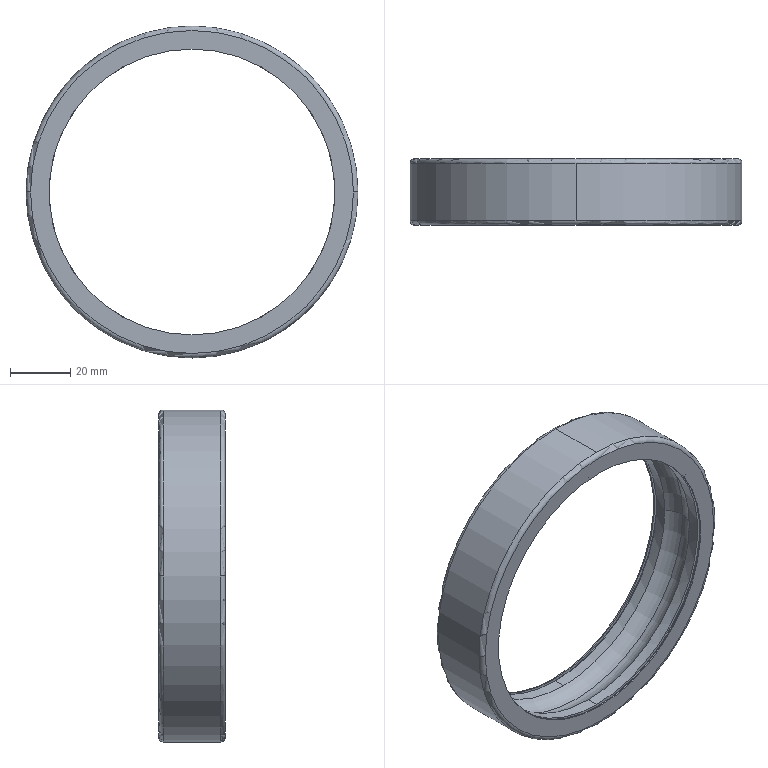Part | SolidWorks | features BaseBody 1 | 1 solid | 28 faces | box 110 x 22 x 110 mm | volume 46776 mm3 | cylinder 14 | torus 8 | plane 6 | commonest cylinder face diameters 94.7 x8 96.7 x4 110 x2
STEP:
#1=CARTESIAN_POINT('',(-2132.95,1024.569,-1530.274));
#2=VERTEX_POINT('',#1);
#3=CARTESIAN_POINT('',(-2132.95,1024.569,-1624.974));
#4=VERTEX_POINT('',#3);
#5=CARTESIAN_POINT('',(-2132.95,1024.569,-1577.624));
#6=DIRECTION('',(0.,-1.,0.));
#7=DIRECTION('',(0.,0.,1.));
#8=AXIS2_PLACEMENT_3D('',#5,#6,#7);
#9=CIRCLE('',#8,47.35);
#10=EDGE_CURVE('',#2,#4,#9,.T.);
#11=ORIENTED_EDGE('',*,*,#10,.F.);
#12=CARTESIAN_POINT('',(-2132.95,1024.569,-1577.624));
#13=DIRECTION('',(0.,-1.,0.));
#14=DIRECTION('',(0.,0.,-1.));
#15=AXIS2_PLACEMENT_3D('',#12,#13,#14);
#16=CIRCLE('',#15,47.35);
#17=EDGE_CURVE('',#4,#2,#16,.T.);
#18=ORIENTED_EDGE('',*,*,#17,.F.);
#19=EDGE_LOOP('',(#11,#18));
#20=FACE_BOUND('',#19,.T.);
#21=CARTESIAN_POINT('',(-2079.45,1024.569,-1577.624));
#22=VERTEX_POINT('',#21);
#23=CARTESIAN_POINT('',(-2186.45,1024.569,-1577.624));
#24=VERTEX_POINT('',#23);
#25=CARTESIAN_POINT('',(-2132.95,1024.569,-1577.624));
#26=DIRECTION('',(0.,-1.,0.));
#27=DIRECTION('',(0.,0.,1.));
#28=AXIS2_PLACEMENT_3D('',#25,#26,#27);
#29=CIRCLE('',#28,53.5);
#30=EDGE_CURVE('',#22,#24,#29,.T.);
#31=ORIENTED_EDGE('',*,*,#30,.T.);
#32=CARTESIAN_POINT('',(-2132.95,1024.569,-1577.624));
#33=DIRECTION('',(0.,-1.,0.));
#34=DIRECTION('',(-1.,0.,0.));
#35=AXIS2_PLACEMENT_3D('',#32,#33,#34);
#36=CIRCLE('',#35,53.5);
#37=EDGE_CURVE('',#24,#22,#36,.T.);
#38=ORIENTED_EDGE('',*,*,#37,.T.);
#39=EDGE_LOOP('',(#31,#38));
#40=FACE_OUTER_BOUND('',#39,.T.);
#41=CARTESIAN_POINT('',(-2074.1,1024.569,-1636.435));
#42=DIRECTION('',(0.,-1.,0.));
#43=DIRECTION('',(0.,0.,-1.));
#44=AXIS2_PLACEMENT_3D('',#41,#42,#43);
#45=PLANE('',#44);
#46=ADVANCED_FACE('',(#20,#40),#45,.T.);
#47=CARTESIAN_POINT('',(-2077.95,1026.069,-1577.624));
#48=VERTEX_POINT('',#47);
#49=CARTESIAN_POINT('',(-2079.45,1026.069,-1577.624));
#50=DIRECTION('',(0.,0.,-1.));
#51=DIRECTION('',(1.,0.,0.));
#52=AXIS2_PLACEMENT_3D('',#49,#50,#51);
#53=CIRCLE('',#52,1.5);
#54=EDGE_CURVE('',#48,#22,#53,.T.);
#55=ORIENTED_EDGE('',*,*,#54,.T.);
#56=ORIENTED_EDGE('',*,*,#37,.F.);
#57=CARTESIAN_POINT('',(-2187.95,1026.069,-1577.624));
#58=VERTEX_POINT('',#57);
#59=CARTESIAN_POINT('',(-2186.45,1026.069,-1577.624));
#60=DIRECTION('',(0.,0.,-1.));
#61=DIRECTION('',(0.,-1.,0.));
#62=AXIS2_PLACEMENT_3D('',#59,#60,#61);
#63=CIRCLE('',#62,1.5);
#64=EDGE_CURVE('',#24,#58,#63,.T.);
#65=ORIENTED_EDGE('',*,*,#64,.T.);
#66=CARTESIAN_POINT('',(-2132.95,1026.069,-1632.624));
#67=VERTEX_POINT('',#66);
#68=CARTESIAN_POINT('',(-2132.95,1026.069,-1577.624));
#69=DIRECTION('',(0.,-1.,0.));
#70=DIRECTION('',(-1.,0.,0.));
#71=AXIS2_PLACEMENT_3D('',#68,#69,#70);
#72=CIRCLE('',#71,55.);
#73=EDGE_CURVE('',#58,#67,#72,.T.);
#74=ORIENTED_EDGE('',*,*,#73,.T.);
#75=CARTESIAN_POINT('',(-2132.95,1026.069,-1577.624));
#76=DIRECTION('',(0.,-1.,0.));
#77=DIRECTION('',(0.,0.,-1.));
#78=AXIS2_PLACEMENT_3D('',#75,#76,#77);
#79=CIRCLE('',#78,55.);
#80=EDGE_CURVE('',#67,#48,#79,.T.);
#81=ORIENTED_EDGE('',*,*,#80,.T.);
#82=EDGE_LOOP('',(#55,#56,#65,#74,#81));
#83=FACE_OUTER_BOUND('',#82,.T.);
#84=CARTESIAN_POINT('',(-2132.95,1026.069,-1577.624));
#85=DIRECTION('',(0.,-1.,0.));
#86=DIRECTION('',(-0.9962,0.,0.08716));
#87=AXIS2_PLACEMENT_3D('',#84,#85,#86);
#88=TOROIDAL_SURFACE('',#87,53.5,1.5);
#89=ADVANCED_FACE('',(#83),#88,.T.);
#90=CARTESIAN_POINT('',(-2132.95,1045.069,-1522.624));
#91=VERTEX_POINT('',#90);
#92=CARTESIAN_POINT('',(-2132.95,1026.069,-1522.624));
#93=VERTEX_POINT('',#92);
#94=CARTESIAN_POINT('',(-2132.95,1045.069,-1522.624));
#95=DIRECTION('',(0.,-1.,0.));
#96=VECTOR('',#95,1000.);
#97=LINE('',#94,#96);
#98=EDGE_CURVE('',#91,#93,#97,.T.);
#99=ORIENTED_EDGE('',*,*,#98,.T.);
#100=CARTESIAN_POINT('',(-2132.95,1026.069,-1577.624));
#101=DIRECTION('',(0.,-1.,0.));
#102=DIRECTION('',(1.,0.,0.));
#103=AXIS2_PLACEMENT_3D('',#100,#101,#102);
#104=CIRCLE('',#103,55.);
#105=EDGE_CURVE('',#48,#93,#104,.T.);
#106=ORIENTED_EDGE('',*,*,#105,.F.);
#107=ORIENTED_EDGE('',*,*,#80,.F.);
#108=CARTESIAN_POINT('',(-2132.95,1045.069,-1632.624));
#109=VERTEX_POINT('',#108);
#110=CARTESIAN_POINT('',(-2132.95,1026.069,-1632.624));
#111=DIRECTION('',(0.,1.,0.));
#112=VECTOR('',#111,1000.);
#113=LINE('',#110,#112);
#114=EDGE_CURVE('',#67,#109,#113,.T.);
#115=ORIENTED_EDGE('',*,*,#114,.T.);
#116=CARTESIAN_POINT('',(-2077.95,1045.069,-1577.624));
#117=VERTEX_POINT('',#116);
#118=CARTESIAN_POINT('',(-2132.95,1045.069,-1577.624));
#119=DIRECTION('',(0.,-1.,0.));
#120=DIRECTION('',(0.,0.,-1.));
#121=AXIS2_PLACEMENT_3D('',#118,#119,#120);
#122=CIRCLE('',#121,55.);
#123=EDGE_CURVE('',#109,#117,#122,.T.);
#124=ORIENTED_EDGE('',*,*,#123,.T.);
#125=CARTESIAN_POINT('',(-2132.95,1045.069,-1577.624));
#126=DIRECTION('',(0.,-1.,0.));
#127=DIRECTION('',(1.,0.,0.));
#128=AXIS2_PLACEMENT_3D('',#125,#126,#127);
#129=CIRCLE('',#128,55.);
#130=EDGE_CURVE('',#117,#91,#129,.T.);
#131=ORIENTED_EDGE('',*,*,#130,.T.);
#132=EDGE_LOOP('',(#99,#106,#107,#115,#124,#131));
#133=FACE_OUTER_BOUND('',#132,.T.);
#134=CARTESIAN_POINT('',(-2132.95,1046.019,-1577.624));
#135=DIRECTION('',(0.,1.,0.));
#136=DIRECTION('',(-0.08716,0.,0.9962));
#137=AXIS2_PLACEMENT_3D('',#134,#135,#136);
#138=CYLINDRICAL_SURFACE('',#137,55.);
#139=ADVANCED_FACE('',(#133),#138,.T.);
#140=CARTESIAN_POINT('',(-2079.45,1046.569,-1577.624));
#141=VERTEX_POINT('',#140);
#142=CARTESIAN_POINT('',(-2079.45,1045.069,-1577.624));
#143=DIRECTION('',(0.,0.,-1.));
#144=DIRECTION('',(0.,1.,0.));
#145=AXIS2_PLACEMENT_3D('',#142,#143,#144);
#146=CIRCLE('',#145,1.5);
#147=EDGE_CURVE('',#141,#117,#146,.T.);
#148=ORIENTED_EDGE('',*,*,#147,.T.);
#149=ORIENTED_EDGE('',*,*,#123,.F.);
#150=CARTESIAN_POINT('',(-2187.95,1045.069,-1577.624));
#151=VERTEX_POINT('',#150);
#152=CARTESIAN_POINT('',(-2132.95,1045.069,-1577.624));
#153=DIRECTION('',(0.,-1.,0.));
#154=DIRECTION('',(-1.,0.,0.));
#155=AXIS2_PLACEMENT_3D('',#152,#153,#154);
#156=CIRCLE('',#155,55.);
#157=EDGE_CURVE('',#151,#109,#156,.T.);
#158=ORIENTED_EDGE('',*,*,#157,.F.);
#159=CARTESIAN_POINT('',(-2186.45,1046.569,-1577.624));
#160=VERTEX_POINT('',#159);
#161=CARTESIAN_POINT('',(-2186.45,1045.069,-1577.624));
#162=DIRECTION('',(0.,0.,-1.));
#163=DIRECTION('',(-1.,0.,0.));
#164=AXIS2_PLACEMENT_3D('',#161,#162,#163);
#165=CIRCLE('',#164,1.5);
#166=EDGE_CURVE('',#151,#160,#165,.T.);
#167=ORIENTED_EDGE('',*,*,#166,.T.);
#168=CARTESIAN_POINT('',(-2132.95,1046.569,-1577.624));
#169=DIRECTION('',(0.,1.,0.));
#170=DIRECTION('',(1.,0.,0.));
#171=AXIS2_PLACEMENT_3D('',#168,#169,#170);
#172=CIRCLE('',#171,53.5);
#173=EDGE_CURVE('',#141,#160,#172,.T.);
#174=ORIENTED_EDGE('',*,*,#173,.F.);
#175=EDGE_LOOP('',(#148,#149,#158,#167,#174));
#176=FACE_OUTER_BOUND('',#175,.T.);
#177=CARTESIAN_POINT('',(-2132.95,1045.069,-1577.624));
#178=DIRECTION('',(0.,-1.,0.));
#179=DIRECTION('',(-0.9962,0.,0.08716));
#180=AXIS2_PLACEMENT_3D('',#177,#178,#179);
#181=TOROIDAL_SURFACE('',#180,53.5,1.5);
#182=ADVANCED_FACE('',(#176),#181,.T.);
#183=CARTESIAN_POINT('',(-2132.95,1046.569,-1624.974));
#184=VERTEX_POINT('',#183);
#185=CARTESIAN_POINT('',(-2132.95,1046.569,-1530.274));
#186=VERTEX_POINT('',#185);
#187=CARTESIAN_POINT('',(-2132.95,1046.569,-1577.624));
#188=DIRECTION('',(0.,1.,0.));
#189=DIRECTION('',(0.,0.,-1.));
#190=AXIS2_PLACEMENT_3D('',#187,#188,#189);
#191=CIRCLE('',#190,47.35);
#192=EDGE_CURVE('',#184,#186,#191,.T.);
#193=ORIENTED_EDGE('',*,*,#192,.F.);
#194=CARTESIAN_POINT('',(-2132.95,1046.569,-1577.624));
#195=DIRECTION('',(0.,1.,0.));
#196=DIRECTION('',(0.,0.,1.));
#197=AXIS2_PLACEMENT_3D('',#194,#195,#196);
#198=CIRCLE('',#197,47.35);
#199=EDGE_CURVE('',#186,#184,#198,.T.);
#200=ORIENTED_EDGE('',*,*,#199,.F.);
#201=EDGE_LOOP('',(#193,#200));
#202=FACE_BOUND('',#201,.T.);
#203=CARTESIAN_POINT('',(-2132.95,1046.569,-1577.624));
#204=DIRECTION('',(0.,1.,0.));
#205=DIRECTION('',(-1.,0.,0.));
#206=AXIS2_PLACEMENT_3D('',#203,#204,#205);
#207=CIRCLE('',#206,53.5);
#208=EDGE_CURVE('',#160,#141,#207,.T.);
#209=ORIENTED_EDGE('',*,*,#208,.T.);
#210=ORIENTED_EDGE('',*,*,#173,.T.);
#211=EDGE_LOOP('',(#209,#210));
#212=FACE_OUTER_BOUND('',#211,.T.);
#213=CARTESIAN_POINT('',(-2074.1,1046.569,-1518.774));
#214=DIRECTION('',(0.,1.,0.));
#215=DIRECTION('',(1.,0.,0.));
#216=AXIS2_PLACEMENT_3D('',#213,#214,#215);
#217=PLANE('',#216);
#218=ADVANCED_FACE('',(#202,#212),#217,.T.);
#219=CARTESIAN_POINT('',(-2132.95,1046.169,-1530.274));
#220=VERTEX_POINT('',#219);
#221=CARTESIAN_POINT('',(-2132.95,1046.569,-1530.274));
#222=DIRECTION('',(0.,-1.,0.));
#223=VECTOR('',#222,1000.);
#224=LINE('',#221,#223);
#225=EDGE_CURVE('',#186,#220,#224,.T.);
#226=ORIENTED_EDGE('',*,*,#225,.T.);
#227=CARTESIAN_POINT('',(-2132.95,1046.169,-1624.974));
#228=VERTEX_POINT('',#227);
#229=CARTESIAN_POINT('',(-2132.95,1046.169,-1577.624));
#230=DIRECTION('',(0.,-1.,0.));
#231=DIRECTION('',(0.,0.,1.));
#232=AXIS2_PLACEMENT_3D('',#229,#230,#231);
#233=CIRCLE('',#232,47.35);
#234=EDGE_CURVE('',#220,#228,#233,.T.);
#235=ORIENTED_EDGE('',*,*,#234,.T.);
#236=CARTESIAN_POINT('',(-2132.95,1046.169,-1624.974));
#237=DIRECTION('',(0.,1.,0.));
#238=VECTOR('',#237,1000.);
#239=LINE('',#236,#238);
#240=EDGE_CURVE('',#228,#184,#239,.T.);
#241=ORIENTED_EDGE('',*,*,#240,.T.);
#242=ORIENTED_EDGE('',*,*,#192,.T.);
#243=EDGE_LOOP('',(#226,#235,#241,#242));
#244=FACE_OUTER_BOUND('',#243,.T.);
#245=CARTESIAN_POINT('',(-2132.95,1046.149,-1577.624));
#246=DIRECTION('',(0.,1.,0.));
#247=DIRECTION('',(0.08716,0.,-0.9962));
#248=AXIS2_PLACEMENT_3D('',#245,#246,#247);
#249=CYLINDRICAL_SURFACE('',#248,47.35);
#250=ADVANCED_FACE('',(#244),#249,.F.);
#251=ORIENTED_EDGE('',*,*,#234,.F.);
#252=CARTESIAN_POINT('',(-2132.95,1046.169,-1577.624));
#253=DIRECTION('',(0.,-1.,0.));
#254=DIRECTION('',(0.,0.,-1.));
#255=AXIS2_PLACEMENT_3D('',#252,#253,#254);
#256=CIRCLE('',#255,47.35);
#257=EDGE_CURVE('',#228,#220,#256,.T.);
#258=ORIENTED_EDGE('',*,*,#257,.F.);
#259=EDGE_LOOP('',(#251,#258));
#260=FACE_BOUND('',#259,.T.);
#261=CARTESIAN_POINT('',(-2132.95,1046.169,-1529.274));
#262=VERTEX_POINT('',#261);
#263=CARTESIAN_POINT('',(-2132.95,1046.169,-1625.974));
#264=VERTEX_POINT('',#263);
#265=CARTESIAN_POINT('',(-2132.95,1046.169,-1577.624));
#266=DIRECTION('',(0.,-1.,0.));
#267=DIRECTION('',(0.,0.,1.));
#268=AXIS2_PLACEMENT_3D('',#265,#266,#267);
#269=CIRCLE('',#268,48.35);
#270=EDGE_CURVE('',#262,#264,#269,.T.);
#271=ORIENTED_EDGE('',*,*,#270,.T.);
#272=CARTESIAN_POINT('',(-2132.95,1046.169,-1577.624));
#273=DIRECTION('',(0.,-1.,0.));
#274=DIRECTION('',(0.,0.,-1.));
#275=AXIS2_PLACEMENT_3D('',#272,#273,#274);
#276=CIRCLE('',#275,48.35);
#277=EDGE_CURVE('',#264,#262,#276,.T.);
#278=ORIENTED_EDGE('',*,*,#277,.T.);
#279=EDGE_LOOP('',(#271,#278));
#280=FACE_OUTER_BOUND('',#279,.T.);
#281=CARTESIAN_POINT('',(-2079.804,1046.169,-1630.809));
#282=DIRECTION('',(0.,-1.,0.));
#283=DIRECTION('',(0.,0.,-1.));
#284=AXIS2_PLACEMENT_3D('',#281,#282,#283);
#285=PLANE('',#284);
#286=ADVANCED_FACE('',(#260,#280),#285,.T.);
#287=CARTESIAN_POINT('',(-2132.95,1045.169,-1529.274));
#288=VERTEX_POINT('',#287);
#289=CARTESIAN_POINT('',(-2132.95,1046.169,-1529.274));
#290=DIRECTION('',(0.,-1.,0.));
#291=VECTOR('',#290,1000.);
#292=LINE('',#289,#291);
#293=EDGE_CURVE('',#262,#288,#292,.T.);
#294=ORIENTED_EDGE('',*,*,#293,.T.);
#295=CARTESIAN_POINT('',(-2132.95,1045.169,-1625.974));
#296=VERTEX_POINT('',#295);
#297=CARTESIAN_POINT('',(-2132.95,1045.169,-1577.624));
#298=DIRECTION('',(0.,1.,0.));
#299=DIRECTION('',(0.,0.,-1.));
#300=AXIS2_PLACEMENT_3D('',#297,#298,#299);
#301=CIRCLE('',#300,48.35);
#302=EDGE_CURVE('',#296,#288,#301,.T.);
#303=ORIENTED_EDGE('',*,*,#302,.F.);
#304=CARTESIAN_POINT('',(-2132.95,1045.169,-1625.974));
#305=DIRECTION('',(0.,1.,0.));
#306=VECTOR('',#305,1000.);
#307=LINE('',#304,#306);
#308=EDGE_CURVE('',#296,#264,#307,.T.);
#309=ORIENTED_EDGE('',*,*,#308,.T.);
#310=ORIENTED_EDGE('',*,*,#270,.F.);
#311=EDGE_LOOP('',(#294,#303,#309,#310));
#312=FACE_OUTER_BOUND('',#311,.T.);
#313=CARTESIAN_POINT('',(-2132.95,1045.119,-1577.624));
#314=DIRECTION('',(0.,1.,0.));
#315=DIRECTION('',(0.08716,0.,-0.9962));
#316=AXIS2_PLACEMENT_3D('',#313,#314,#315);
#317=CYLINDRICAL_SURFACE('',#316,48.35);
#318=ADVANCED_FACE('',(#312),#317,.F.);
#319=CARTESIAN_POINT('',(-2132.95,1045.169,-1624.974));
#320=VERTEX_POINT('',#319);
#321=CARTESIAN_POINT('',(-2132.95,1045.169,-1530.274));
#322=VERTEX_POINT('',#321);
#323=CARTESIAN_POINT('',(-2132.95,1045.169,-1577.624));
#324=DIRECTION('',(0.,1.,0.));
#325=DIRECTION('',(0.,0.,-1.));
#326=AXIS2_PLACEMENT_3D('',#323,#324,#325);
#327=CIRCLE('',#326,47.35);
#328=EDGE_CURVE('',#320,#322,#327,.T.);
#329=ORIENTED_EDGE('',*,*,#328,.F.);
#330=CARTESIAN_POINT('',(-2132.95,1045.169,-1577.624));
#331=DIRECTION('',(0.,1.,0.));
#332=DIRECTION('',(0.,0.,1.));
#333=AXIS2_PLACEMENT_3D('',#330,#331,#332);
#334=CIRCLE('',#333,47.35);
#335=EDGE_CURVE('',#322,#320,#334,.T.);
#336=ORIENTED_EDGE('',*,*,#335,.F.);
#337=EDGE_LOOP('',(#329,#336));
#338=FACE_BOUND('',#337,.T.);
#339=ORIENTED_EDGE('',*,*,#302,.T.);
#340=CARTESIAN_POINT('',(-2132.95,1045.169,-1577.624));
#341=DIRECTION('',(0.,1.,0.));
#342=DIRECTION('',(0.,0.,1.));
#343=AXIS2_PLACEMENT_3D('',#340,#341,#342);
#344=CIRCLE('',#343,48.35);
#345=EDGE_CURVE('',#288,#296,#344,.T.);
#346=ORIENTED_EDGE('',*,*,#345,.T.);
#347=EDGE_LOOP('',(#339,#346));
#348=FACE_OUTER_BOUND('',#347,.T.);
#349=CARTESIAN_POINT('',(-2079.804,1045.169,-1524.439));
#350=DIRECTION('',(0.,1.,0.));
#351=DIRECTION('',(1.,0.,0.));
#352=AXIS2_PLACEMENT_3D('',#349,#350,#351);
#353=PLANE('',#352);
#354=ADVANCED_FACE('',(#338,#348),#353,.T.);
#355=CARTESIAN_POINT('',(-2132.95,1041.289,-1530.274));
#356=VERTEX_POINT('',#355);
#357=CARTESIAN_POINT('',(-2132.95,1045.169,-1530.274));
#358=DIRECTION('',(0.,-1.,0.));
#359=VECTOR('',#358,1000.);
#360=LINE('',#357,#359);
#361=EDGE_CURVE('',#322,#356,#360,.T.);
#362=ORIENTED_EDGE('',*,*,#361,.T.);
#363=CARTESIAN_POINT('',(-2180.3,1041.289,-1577.624));
#364=VERTEX_POINT('',#363);
#365=CARTESIAN_POINT('',(-2132.95,1041.289,-1577.624));
#366=DIRECTION('',(0.,-1.,0.));
#367=DIRECTION('',(0.,0.,1.));
#368=AXIS2_PLACEMENT_3D('',#365,#366,#367);
#369=CIRCLE('',#368,47.35);
#370=EDGE_CURVE('',#356,#364,#369,.T.);
#371=ORIENTED_EDGE('',*,*,#370,.T.);
#372=CARTESIAN_POINT('',(-2132.95,1041.289,-1624.974));
#373=VERTEX_POINT('',#372);
#374=CARTESIAN_POINT('',(-2132.95,1041.289,-1577.624));
#375=DIRECTION('',(0.,-1.,0.));
#376=DIRECTION('',(-1.,0.,0.));
#377=AXIS2_PLACEMENT_3D('',#374,#375,#376);
#378=CIRCLE('',#377,47.35);
#379=EDGE_CURVE('',#364,#373,#378,.T.);
#380=ORIENTED_EDGE('',*,*,#379,.T.);
#381=CARTESIAN_POINT('',(-2132.95,1041.289,-1624.974));
#382=DIRECTION('',(0.,1.,0.));
#383=VECTOR('',#382,1000.);
#384=LINE('',#381,#383);
#385=EDGE_CURVE('',#373,#320,#384,.T.);
#386=ORIENTED_EDGE('',*,*,#385,.T.);
#387=ORIENTED_EDGE('',*,*,#328,.T.);
#388=EDGE_LOOP('',(#362,#371,#380,#386,#387));
#389=FACE_OUTER_BOUND('',#388,.T.);
#390=CARTESIAN_POINT('',(-2132.95,1041.095,-1577.624));
#391=DIRECTION('',(0.,1.,0.));
#392=DIRECTION('',(0.08716,0.,-0.9962));
#393=AXIS2_PLACEMENT_3D('',#390,#391,#392);
#394=CYLINDRICAL_SURFACE('',#393,47.35);
#395=ADVANCED_FACE('',(#389),#394,.F.);
#396=CARTESIAN_POINT('',(-2082.95,1035.569,-1577.624));
#397=VERTEX_POINT('',#396);
#398=CARTESIAN_POINT('',(-2182.95,1035.569,-1577.624));
#399=VERTEX_POINT('',#398);
#400=CARTESIAN_POINT('',(-2132.95,1035.569,-1577.624));
#401=DIRECTION('',(0.,-1.,0.));
#402=DIRECTION('',(1.,0.,0.));
#403=AXIS2_PLACEMENT_3D('',#400,#401,#402);
#404=CIRCLE('',#403,50.);
#405=EDGE_CURVE('',#397,#399,#404,.T.);
#406=ORIENTED_EDGE('',*,*,#405,.T.);
#407=CARTESIAN_POINT('',(-2175.45,1035.569,-1577.624));
#408=DIRECTION('',(0.,0.,-1.));
#409=DIRECTION('',(-1.,0.,0.));
#410=AXIS2_PLACEMENT_3D('',#407,#408,#409);
#411=CIRCLE('',#410,7.5);
#412=EDGE_CURVE('',#399,#364,#411,.T.);
#413=ORIENTED_EDGE('',*,*,#412,.T.);
#414=ORIENTED_EDGE('',*,*,#370,.F.);
#415=CARTESIAN_POINT('',(-2085.6,1041.289,-1577.624));
#416=VERTEX_POINT('',#415);
#417=CARTESIAN_POINT('',(-2132.95,1041.289,-1577.624));
#418=DIRECTION('',(0.,-1.,0.));
#419=DIRECTION('',(1.,0.,0.));
#420=AXIS2_PLACEMENT_3D('',#417,#418,#419);
#421=CIRCLE('',#420,47.35);
#422=EDGE_CURVE('',#416,#356,#421,.T.);
#423=ORIENTED_EDGE('',*,*,#422,.F.);
#424=CARTESIAN_POINT('',(-2090.45,1035.569,-1577.624));
#425=DIRECTION('',(0.,0.,-1.));
#426=DIRECTION('',(0.6467,0.7628,0.));
#427=AXIS2_PLACEMENT_3D('',#424,#425,#426);
#428=CIRCLE('',#427,7.5);
#429=EDGE_CURVE('',#416,#397,#428,.T.);
#430=ORIENTED_EDGE('',*,*,#429,.T.);
#431=EDGE_LOOP('',(#406,#413,#414,#423,#430));
#432=FACE_OUTER_BOUND('',#431,.T.);
#433=CARTESIAN_POINT('',(-2132.95,1035.569,-1577.624));
#434=DIRECTION('',(0.,-1.,0.));
#435=DIRECTION('',(0.9962,0.,-0.08716));
#436=AXIS2_PLACEMENT_3D('',#433,#434,#435);
#437=TOROIDAL_SURFACE('',#436,42.5,7.5);
#438=ADVANCED_FACE('',(#432),#437,.F.);
#439=CARTESIAN_POINT('',(-2132.95,1029.848,-1530.274));
#440=VERTEX_POINT('',#439);
#441=CARTESIAN_POINT('',(-2132.95,1025.969,-1530.274));
#442=VERTEX_POINT('',#441);
#443=CARTESIAN_POINT('',(-2132.95,1029.848,-1530.274));
#444=DIRECTION('',(0.,-1.,0.));
#445=VECTOR('',#444,1000.);
#446=LINE('',#443,#445);
#447=EDGE_CURVE('',#440,#442,#446,.T.);
#448=ORIENTED_EDGE('',*,*,#447,.T.);
#449=CARTESIAN_POINT('',(-2132.95,1025.969,-1624.974));
#450=VERTEX_POINT('',#449);
#451=CARTESIAN_POINT('',(-2132.95,1025.969,-1577.624));
#452=DIRECTION('',(0.,-1.,0.));
#453=DIRECTION('',(0.,0.,1.));
#454=AXIS2_PLACEMENT_3D('',#451,#452,#453);
#455=CIRCLE('',#454,47.35);
#456=EDGE_CURVE('',#442,#450,#455,.T.);
#457=ORIENTED_EDGE('',*,*,#456,.T.);
#458=CARTESIAN_POINT('',(-2132.95,1029.848,-1624.974));
#459=VERTEX_POINT('',#458);
#460=CARTESIAN_POINT('',(-2132.95,1025.969,-1624.974));
#461=DIRECTION('',(0.,1.,0.));
#462=VECTOR('',#461,1000.);
#463=LINE('',#460,#462);
#464=EDGE_CURVE('',#450,#459,#463,.T.);
#465=ORIENTED_EDGE('',*,*,#464,.T.);
#466=CARTESIAN_POINT('',(-2180.3,1029.848,-1577.624));
#467=VERTEX_POINT('',#466);
#468=CARTESIAN_POINT('',(-2132.95,1029.848,-1577.624));
#469=DIRECTION('',(0.,-1.,0.));
#470=DIRECTION('',(-1.,0.,0.));
#471=AXIS2_PLACEMENT_3D('',#468,#469,#470);
#472=CIRCLE('',#471,47.35);
#473=EDGE_CURVE('',#467,#459,#472,.T.);
#474=ORIENTED_EDGE('',*,*,#473,.F.);
#475=CARTESIAN_POINT('',(-2132.95,1029.848,-1577.624));
#476=DIRECTION('',(0.,-1.,0.));
#477=DIRECTION('',(0.,0.,1.));
#478=AXIS2_PLACEMENT_3D('',#475,#476,#477);
#479=CIRCLE('',#478,47.35);
#480=EDGE_CURVE('',#440,#467,#479,.T.);
#481=ORIENTED_EDGE('',*,*,#480,.F.);
#482=EDGE_LOOP('',(#448,#457,#465,#474,#481));
#483=FACE_OUTER_BOUND('',#482,.T.);
#484=CARTESIAN_POINT('',(-2132.95,1025.775,-1577.624));
#485=DIRECTION('',(0.,1.,0.));
#486=DIRECTION('',(0.08716,0.,-0.9962));
#487=AXIS2_PLACEMENT_3D('',#484,#485,#486);
#488=CYLINDRICAL_SURFACE('',#487,47.35);
#489=ADVANCED_FACE('',(#483),#488,.F.);
#490=ORIENTED_EDGE('',*,*,#456,.F.);
#491=CARTESIAN_POINT('',(-2132.95,1025.969,-1577.624));
#492=DIRECTION('',(0.,-1.,0.));
#493=DIRECTION('',(0.,0.,-1.));
#494=AXIS2_PLACEMENT_3D('',#491,#492,#493);
#495=CIRCLE('',#494,47.35);
#496=EDGE_CURVE('',#450,#442,#495,.T.);
#497=ORIENTED_EDGE('',*,*,#496,.F.);
#498=EDGE_LOOP('',(#490,#497));
#499=FACE_BOUND('',#498,.T.);
#500=CARTESIAN_POINT('',(-2132.95,1025.969,-1529.274));
#501=VERTEX_POINT('',#500);
#502=CARTESIAN_POINT('',(-2132.95,1025.969,-1625.974));
#503=VERTEX_POINT('',#502);
#504=CARTESIAN_POINT('',(-2132.95,1025.969,-1577.624));
#505=DIRECTION('',(0.,-1.,0.));
#506=DIRECTION('',(0.,0.,1.));
#507=AXIS2_PLACEMENT_3D('',#504,#505,#506);
#508=CIRCLE('',#507,48.35);
#509=EDGE_CURVE('',#501,#503,#508,.T.);
#510=ORIENTED_EDGE('',*,*,#509,.T.);
#511=CARTESIAN_POINT('',(-2132.95,1025.969,-1577.624));
#512=DIRECTION('',(0.,-1.,0.));
#513=DIRECTION('',(0.,0.,-1.));
#514=AXIS2_PLACEMENT_3D('',#511,#512,#513);
#515=CIRCLE('',#514,48.35);
#516=EDGE_CURVE('',#503,#501,#515,.T.);
#517=ORIENTED_EDGE('',*,*,#516,.T.);
#518=EDGE_LOOP('',(#510,#517));
#519=FACE_OUTER_BOUND('',#518,.T.);
#520=CARTESIAN_POINT('',(-2079.804,1025.969,-1630.809));
#521=DIRECTION('',(0.,-1.,0.));
#522=DIRECTION('',(0.,0.,-1.));
#523=AXIS2_PLACEMENT_3D('',#520,#521,#522);
#524=PLANE('',#523);
#525=ADVANCED_FACE('',(#499,#519),#524,.T.);
#526=CARTESIAN_POINT('',(-2132.95,1024.969,-1529.274));
#527=VERTEX_POINT('',#526);
#528=CARTESIAN_POINT('',(-2132.95,1025.969,-1529.274));
#529=DIRECTION('',(0.,-1.,0.));
#530=VECTOR('',#529,1000.);
#531=LINE('',#528,#530);
#532=EDGE_CURVE('',#501,#527,#531,.T.);
#533=ORIENTED_EDGE('',*,*,#532,.T.);
#534=CARTESIAN_POINT('',(-2132.95,1024.969,-1625.974));
#535=VERTEX_POINT('',#534);
#536=CARTESIAN_POINT('',(-2132.95,1024.969,-1577.624));
#537=DIRECTION('',(0.,1.,0.));
#538=DIRECTION('',(0.,0.,-1.));
#539=AXIS2_PLACEMENT_3D('',#536,#537,#538);
#540=CIRCLE('',#539,48.35);
#541=EDGE_CURVE('',#535,#527,#540,.T.);
#542=ORIENTED_EDGE('',*,*,#541,.F.);
#543=CARTESIAN_POINT('',(-2132.95,1024.969,-1625.974));
#544=DIRECTION('',(0.,1.,0.));
#545=VECTOR('',#544,1000.);
#546=LINE('',#543,#545);
#547=EDGE_CURVE('',#535,#503,#546,.T.);
#548=ORIENTED_EDGE('',*,*,#547,.T.);
#549=ORIENTED_EDGE('',*,*,#509,.F.);
#550=EDGE_LOOP('',(#533,#542,#548,#549));
#551=FACE_OUTER_BOUND('',#550,.T.);
#552=CARTESIAN_POINT('',(-2132.95,1024.919,-1577.624));
#553=DIRECTION('',(0.,1.,0.));
#554=DIRECTION('',(0.08716,0.,-0.9962));
#555=AXIS2_PLACEMENT_3D('',#552,#553,#554);
#556=CYLINDRICAL_SURFACE('',#555,48.35);
#557=ADVANCED_FACE('',(#551),#556,.F.);
#558=CARTESIAN_POINT('',(-2132.95,1024.969,-1624.974));
#559=VERTEX_POINT('',#558);
#560=CARTESIAN_POINT('',(-2132.95,1024.969,-1530.274));
#561=VERTEX_POINT('',#560);
#562=CARTESIAN_POINT('',(-2132.95,1024.969,-1577.624));
#563=DIRECTION('',(0.,1.,0.));
#564=DIRECTION('',(0.,0.,-1.));
#565=AXIS2_PLACEMENT_3D('',#562,#563,#564);
#566=CIRCLE('',#565,47.35);
#567=EDGE_CURVE('',#559,#561,#566,.T.);
#568=ORIENTED_EDGE('',*,*,#567,.F.);
#569=CARTESIAN_POINT('',(-2132.95,1024.969,-1577.624));
#570=DIRECTION('',(0.,1.,0.));
#571=DIRECTION('',(0.,0.,1.));
#572=AXIS2_PLACEMENT_3D('',#569,#570,#571);
#573=CIRCLE('',#572,47.35);
#574=EDGE_CURVE('',#561,#559,#573,.T.);
#575=ORIENTED_EDGE('',*,*,#574,.F.);
#576=EDGE_LOOP('',(#568,#575));
#577=FACE_BOUND('',#576,.T.);
#578=ORIENTED_EDGE('',*,*,#541,.T.);
#579=CARTESIAN_POINT('',(-2132.95,1024.969,-1577.624));
#580=DIRECTION('',(0.,1.,0.));
#581=DIRECTION('',(0.,0.,1.));
#582=AXIS2_PLACEMENT_3D('',#579,#580,#581);
#583=CIRCLE('',#582,48.35);
#584=EDGE_CURVE('',#527,#535,#583,.T.);
#585=ORIENTED_EDGE('',*,*,#584,.T.);
#586=EDGE_LOOP('',(#578,#585));
#587=FACE_OUTER_BOUND('',#586,.T.);
#588=CARTESIAN_POINT('',(-2079.804,1024.969,-1524.439));
#589=DIRECTION('',(0.,1.,0.));
#590=DIRECTION('',(1.,0.,0.));
#591=AXIS2_PLACEMENT_3D('',#588,#589,#590);
#592=PLANE('',#591);
#593=ADVANCED_FACE('',(#577,#587),#592,.T.);
#594=CARTESIAN_POINT('',(-2132.95,1024.969,-1530.274));
#595=DIRECTION('',(0.,-1.,0.));
#596=VECTOR('',#595,1000.);
#597=LINE('',#594,#596);
#598=EDGE_CURVE('',#561,#2,#597,.T.);
#599=ORIENTED_EDGE('',*,*,#598,.T.);
#600=ORIENTED_EDGE('',*,*,#10,.T.);
#601=CARTESIAN_POINT('',(-2132.95,1024.569,-1624.974));
#602=DIRECTION('',(0.,1.,0.));
#603=VECTOR('',#602,1000.);
#604=LINE('',#601,#603);
#605=EDGE_CURVE('',#4,#559,#604,.T.);
#606=ORIENTED_EDGE('',*,*,#605,.T.);
#607=ORIENTED_EDGE('',*,*,#567,.T.);
#608=EDGE_LOOP('',(#599,#600,#606,#607));
#609=FACE_OUTER_BOUND('',#608,.T.);
#610=CARTESIAN_POINT('',(-2132.95,1024.549,-1577.624));
#611=DIRECTION('',(0.,1.,0.));
#612=DIRECTION('',(0.08716,0.,-0.9962));
#613=AXIS2_PLACEMENT_3D('',#610,#611,#612);
#614=CYLINDRICAL_SURFACE('',#613,47.35);
#615=ADVANCED_FACE('',(#609),#614,.F.);
#616=ORIENTED_EDGE('',*,*,#598,.F.);
#617=ORIENTED_EDGE('',*,*,#574,.T.);
#618=ORIENTED_EDGE('',*,*,#605,.F.);
#619=ORIENTED_EDGE('',*,*,#17,.T.);
#620=EDGE_LOOP('',(#616,#617,#618,#619));
#621=FACE_OUTER_BOUND('',#620,.T.);
#622=CARTESIAN_POINT('',(-2132.95,1024.549,-1577.624));
#623=DIRECTION('',(0.,1.,0.));
#624=DIRECTION('',(-0.08716,0.,0.9962));
#625=AXIS2_PLACEMENT_3D('',#622,#623,#624);
#626=CYLINDRICAL_SURFACE('',#625,47.35);
#627=ADVANCED_FACE('',(#621),#626,.F.);
#628=ORIENTED_EDGE('',*,*,#532,.F.);
#629=ORIENTED_EDGE('',*,*,#516,.F.);
#630=ORIENTED_EDGE('',*,*,#547,.F.);
#631=ORIENTED_EDGE('',*,*,#584,.F.);
#632=EDGE_LOOP('',(#628,#629,#630,#631));
#633=FACE_OUTER_BOUND('',#632,.T.);
#634=CARTESIAN_POINT('',(-2132.95,1024.919,-1577.624));
#635=DIRECTION('',(0.,1.,0.));
#636=DIRECTION('',(-0.08716,0.,0.9962));
#637=AXIS2_PLACEMENT_3D('',#634,#635,#636);
#638=CYLINDRICAL_SURFACE('',#637,48.35);
#639=ADVANCED_FACE('',(#633),#638,.F.);
#640=ORIENTED_EDGE('',*,*,#447,.F.);
#641=CARTESIAN_POINT('',(-2085.6,1029.848,-1577.624));
#642=VERTEX_POINT('',#641);
#643=CARTESIAN_POINT('',(-2132.95,1029.848,-1577.624));
#644=DIRECTION('',(0.,-1.,0.));
#645=DIRECTION('',(1.,0.,0.));
#646=AXIS2_PLACEMENT_3D('',#643,#644,#645);
#647=CIRCLE('',#646,47.35);
#648=EDGE_CURVE('',#642,#440,#647,.T.);
#649=ORIENTED_EDGE('',*,*,#648,.F.);
#650=CARTESIAN_POINT('',(-2132.95,1029.848,-1577.624));
#651=DIRECTION('',(0.,-1.,0.));
#652=DIRECTION('',(0.,0.,-1.));
#653=AXIS2_PLACEMENT_3D('',#650,#651,#652);
#654=CIRCLE('',#653,47.35);
#655=EDGE_CURVE('',#459,#642,#654,.T.);
#656=ORIENTED_EDGE('',*,*,#655,.F.);
#657=ORIENTED_EDGE('',*,*,#464,.F.);
#658=ORIENTED_EDGE('',*,*,#496,.T.);
#659=EDGE_LOOP('',(#640,#649,#656,#657,#658));
#660=FACE_OUTER_BOUND('',#659,.T.);
#661=CARTESIAN_POINT('',(-2132.95,1025.775,-1577.624));
#662=DIRECTION('',(0.,1.,0.));
#663=DIRECTION('',(-0.08716,0.,0.9962));
#664=AXIS2_PLACEMENT_3D('',#661,#662,#663);
#665=CYLINDRICAL_SURFACE('',#664,47.35);
#666=ADVANCED_FACE('',(#660),#665,.F.);
#667=CARTESIAN_POINT('',(-2132.95,1035.569,-1577.624));
#668=DIRECTION('',(0.,-1.,0.));
#669=DIRECTION('',(-1.,0.,0.));
#670=AXIS2_PLACEMENT_3D('',#667,#668,#669);
#671=CIRCLE('',#670,50.);
#672=EDGE_CURVE('',#399,#397,#671,.T.);
#673=ORIENTED_EDGE('',*,*,#672,.T.);
#674=ORIENTED_EDGE('',*,*,#429,.F.);
#675=CARTESIAN_POINT('',(-2132.95,1041.289,-1577.624));
#676=DIRECTION('',(0.,-1.,0.));
#677=DIRECTION('',(0.,0.,-1.));
#678=AXIS2_PLACEMENT_3D('',#675,#676,#677);
#679=CIRCLE('',#678,47.35);
#680=EDGE_CURVE('',#373,#416,#679,.T.);
#681=ORIENTED_EDGE('',*,*,#680,.F.);
#682=ORIENTED_EDGE('',*,*,#379,.F.);
#683=ORIENTED_EDGE('',*,*,#412,.F.);
#684=EDGE_LOOP('',(#673,#674,#681,#682,#683));
#685=FACE_OUTER_BOUND('',#684,.T.);
#686=CARTESIAN_POINT('',(-2132.95,1035.569,-1577.624));
#687=DIRECTION('',(0.,-1.,0.));
#688=DIRECTION('',(-0.9962,0.,0.08716));
#689=AXIS2_PLACEMENT_3D('',#686,#687,#688);
#690=TOROIDAL_SURFACE('',#689,42.5,7.5);
#691=ADVANCED_FACE('',(#685),#690,.F.);
#692=ORIENTED_EDGE('',*,*,#361,.F.);
#693=ORIENTED_EDGE('',*,*,#335,.T.);
#694=ORIENTED_EDGE('',*,*,#385,.F.);
#695=ORIENTED_EDGE('',*,*,#680,.T.);
#696=ORIENTED_EDGE('',*,*,#422,.T.);
#697=EDGE_LOOP('',(#692,#693,#694,#695,#696));
#698=FACE_OUTER_BOUND('',#697,.T.);
#699=CARTESIAN_POINT('',(-2132.95,1041.095,-1577.624));
#700=DIRECTION('',(0.,1.,0.));
#701=DIRECTION('',(-0.08716,0.,0.9962));
#702=AXIS2_PLACEMENT_3D('',#699,#700,#701);
#703=CYLINDRICAL_SURFACE('',#702,47.35);
#704=ADVANCED_FACE('',(#698),#703,.F.);
#705=ORIENTED_EDGE('',*,*,#293,.F.);
#706=ORIENTED_EDGE('',*,*,#277,.F.);
#707=ORIENTED_EDGE('',*,*,#308,.F.);
#708=ORIENTED_EDGE('',*,*,#345,.F.);
#709=EDGE_LOOP('',(#705,#706,#707,#708));
#710=FACE_OUTER_BOUND('',#709,.T.);
#711=CARTESIAN_POINT('',(-2132.95,1045.119,-1577.624));
#712=DIRECTION('',(0.,1.,0.));
#713=DIRECTION('',(-0.08716,0.,0.9962));
#714=AXIS2_PLACEMENT_3D('',#711,#712,#713);
#715=CYLINDRICAL_SURFACE('',#714,48.35);
#716=ADVANCED_FACE('',(#710),#715,.F.);
#717=ORIENTED_EDGE('',*,*,#225,.F.);
#718=ORIENTED_EDGE('',*,*,#199,.T.);
#719=ORIENTED_EDGE('',*,*,#240,.F.);
#720=ORIENTED_EDGE('',*,*,#257,.T.);
#721=EDGE_LOOP('',(#717,#718,#719,#720));
#722=FACE_OUTER_BOUND('',#721,.T.);
#723=CARTESIAN_POINT('',(-2132.95,1046.149,-1577.624));
#724=DIRECTION('',(0.,1.,0.));
#725=DIRECTION('',(-0.08716,0.,0.9962));
#726=AXIS2_PLACEMENT_3D('',#723,#724,#725);
#727=CYLINDRICAL_SURFACE('',#726,47.35);
#728=ADVANCED_FACE('',(#722),#727,.F.);
#729=ORIENTED_EDGE('',*,*,#147,.F.);
#730=ORIENTED_EDGE('',*,*,#208,.F.);
#731=ORIENTED_EDGE('',*,*,#166,.F.);
#732=CARTESIAN_POINT('',(-2132.95,1045.069,-1577.624));
#733=DIRECTION('',(0.,-1.,0.));
#734=DIRECTION('',(0.,0.,1.));
#735=AXIS2_PLACEMENT_3D('',#732,#733,#734);
#736=CIRCLE('',#735,55.);
#737=EDGE_CURVE('',#91,#151,#736,.T.);
#738=ORIENTED_EDGE('',*,*,#737,.F.);
#739=ORIENTED_EDGE('',*,*,#130,.F.);
#740=EDGE_LOOP('',(#729,#730,#731,#738,#739));
#741=FACE_OUTER_BOUND('',#740,.T.);
#742=CARTESIAN_POINT('',(-2132.95,1045.069,-1577.624));
#743=DIRECTION('',(0.,-1.,0.));
#744=DIRECTION('',(0.9962,0.,-0.08716));
#745=AXIS2_PLACEMENT_3D('',#742,#743,#744);
#746=TOROIDAL_SURFACE('',#745,53.5,1.5);
#747=ADVANCED_FACE('',(#741),#746,.T.);
#748=ORIENTED_EDGE('',*,*,#98,.F.);
#749=ORIENTED_EDGE('',*,*,#737,.T.);
#750=ORIENTED_EDGE('',*,*,#157,.T.);
#751=ORIENTED_EDGE('',*,*,#114,.F.);
#752=ORIENTED_EDGE('',*,*,#73,.F.);
#753=CARTESIAN_POINT('',(-2132.95,1026.069,-1577.624));
#754=DIRECTION('',(0.,-1.,0.));
#755=DIRECTION('',(0.,0.,1.));
#756=AXIS2_PLACEMENT_3D('',#753,#754,#755);
#757=CIRCLE('',#756,55.);
#758=EDGE_CURVE('',#93,#58,#757,.T.);
#759=ORIENTED_EDGE('',*,*,#758,.F.);
#760=EDGE_LOOP('',(#748,#749,#750,#751,#752,#759));
#761=FACE_OUTER_BOUND('',#760,.T.);
#762=CARTESIAN_POINT('',(-2132.95,1046.019,-1577.624));
#763=DIRECTION('',(0.,1.,0.));
#764=DIRECTION('',(0.08716,0.,-0.9962));
#765=AXIS2_PLACEMENT_3D('',#762,#763,#764);
#766=CYLINDRICAL_SURFACE('',#765,55.);
#767=ADVANCED_FACE('',(#761),#766,.T.);
#768=ORIENTED_EDGE('',*,*,#54,.F.);
#769=ORIENTED_EDGE('',*,*,#105,.T.);
#770=ORIENTED_EDGE('',*,*,#758,.T.);
#771=ORIENTED_EDGE('',*,*,#64,.F.);
#772=ORIENTED_EDGE('',*,*,#30,.F.);
#773=EDGE_LOOP('',(#768,#769,#770,#771,#772));
#774=FACE_OUTER_BOUND('',#773,.T.);
#775=CARTESIAN_POINT('',(-2132.95,1026.069,-1577.624));
#776=DIRECTION('',(0.,-1.,0.));
#777=DIRECTION('',(0.9962,0.,-0.08716));
#778=AXIS2_PLACEMENT_3D('',#775,#776,#777);
#779=TOROIDAL_SURFACE('',#778,53.5,1.5);
#780=ADVANCED_FACE('',(#774),#779,.T.);
#781=ORIENTED_EDGE('',*,*,#672,.F.);
#782=CARTESIAN_POINT('',(-2175.45,1035.569,-1577.624));
#783=DIRECTION('',(0.,0.,-1.));
#784=DIRECTION('',(-0.6467,-0.7628,0.));
#785=AXIS2_PLACEMENT_3D('',#782,#783,#784);
#786=CIRCLE('',#785,7.5);
#787=EDGE_CURVE('',#467,#399,#786,.T.);
#788=ORIENTED_EDGE('',*,*,#787,.F.);
#789=ORIENTED_EDGE('',*,*,#473,.T.);
#790=ORIENTED_EDGE('',*,*,#655,.T.);
#791=CARTESIAN_POINT('',(-2090.45,1035.569,-1577.624));
#792=DIRECTION('',(0.,0.,-1.));
#793=DIRECTION('',(1.,0.,0.));
#794=AXIS2_PLACEMENT_3D('',#791,#792,#793);
#795=CIRCLE('',#794,7.5);
#796=EDGE_CURVE('',#397,#642,#795,.T.);
#797=ORIENTED_EDGE('',*,*,#796,.F.);
#798=EDGE_LOOP('',(#781,#788,#789,#790,#797));
#799=FACE_OUTER_BOUND('',#798,.T.);
#800=CARTESIAN_POINT('',(-2132.95,1035.569,-1577.624));
#801=DIRECTION('',(0.,-1.,0.));
#802=DIRECTION('',(-0.9962,0.,0.08716));
#803=AXIS2_PLACEMENT_3D('',#800,#801,#802);
#804=TOROIDAL_SURFACE('',#803,42.5,7.5);
#805=ADVANCED_FACE('',(#799),#804,.F.);
#806=ORIENTED_EDGE('',*,*,#405,.F.);
#807=ORIENTED_EDGE('',*,*,#796,.T.);
#808=ORIENTED_EDGE('',*,*,#648,.T.);
#809=ORIENTED_EDGE('',*,*,#480,.T.);
#810=ORIENTED_EDGE('',*,*,#787,.T.);
#811=EDGE_LOOP('',(#806,#807,#808,#809,#810));
#812=FACE_OUTER_BOUND('',#811,.T.);
#813=CARTESIAN_POINT('',(-2132.95,1035.569,-1577.624));
#814=DIRECTION('',(0.,-1.,0.));
#815=DIRECTION('',(0.9962,0.,-0.08716));
#816=AXIS2_PLACEMENT_3D('',#813,#814,#815);
#817=TOROIDAL_SURFACE('',#816,42.5,7.5);
#818=ADVANCED_FACE('',(#812),#817,.F.);
#819=CLOSED_SHELL('',(#46,#89,#139,#182,#218,#250,#286,#318,#354,#395,#438,#489,#525,#557,#593,#615,#627,#639,#666,#691,#704,#716,#728,#747,#767,#780,#805,#818));
#820=MANIFOLD_SOLID_BREP('',#819);
#821=CARTESIAN_POINT('',(0.,0.,0.));
#822=DIRECTION('',(0.,0.,1.));
#823=DIRECTION('',(1.,0.,0.));
#824=AXIS2_PLACEMENT_3D('',#821,#822,#823);
#825=(LENGTH_UNIT()NAMED_UNIT(*)SI_UNIT(.MILLI.,.METRE.));
#826=UNCERTAINTY_MEASURE_WITH_UNIT(LENGTH_MEASURE(0.00001),#825,'','');
#827=(NAMED_UNIT(*)PLANE_ANGLE_UNIT()SI_UNIT($,.RADIAN.));
#828=(NAMED_UNIT(*)SI_UNIT($,.STERADIAN.)SOLID_ANGLE_UNIT());
#829=(GEOMETRIC_REPRESENTATION_CONTEXT(3)GLOBAL_UNCERTAINTY_ASSIGNED_CONTEXT((#826))GLOBAL_UNIT_ASSIGNED_CONTEXT((#825,#827,#828))REPRESENTATION_CONTEXT('',''));
#830=ADVANCED_BREP_SHAPE_REPRESENTATION('',(#820,#824),#829);